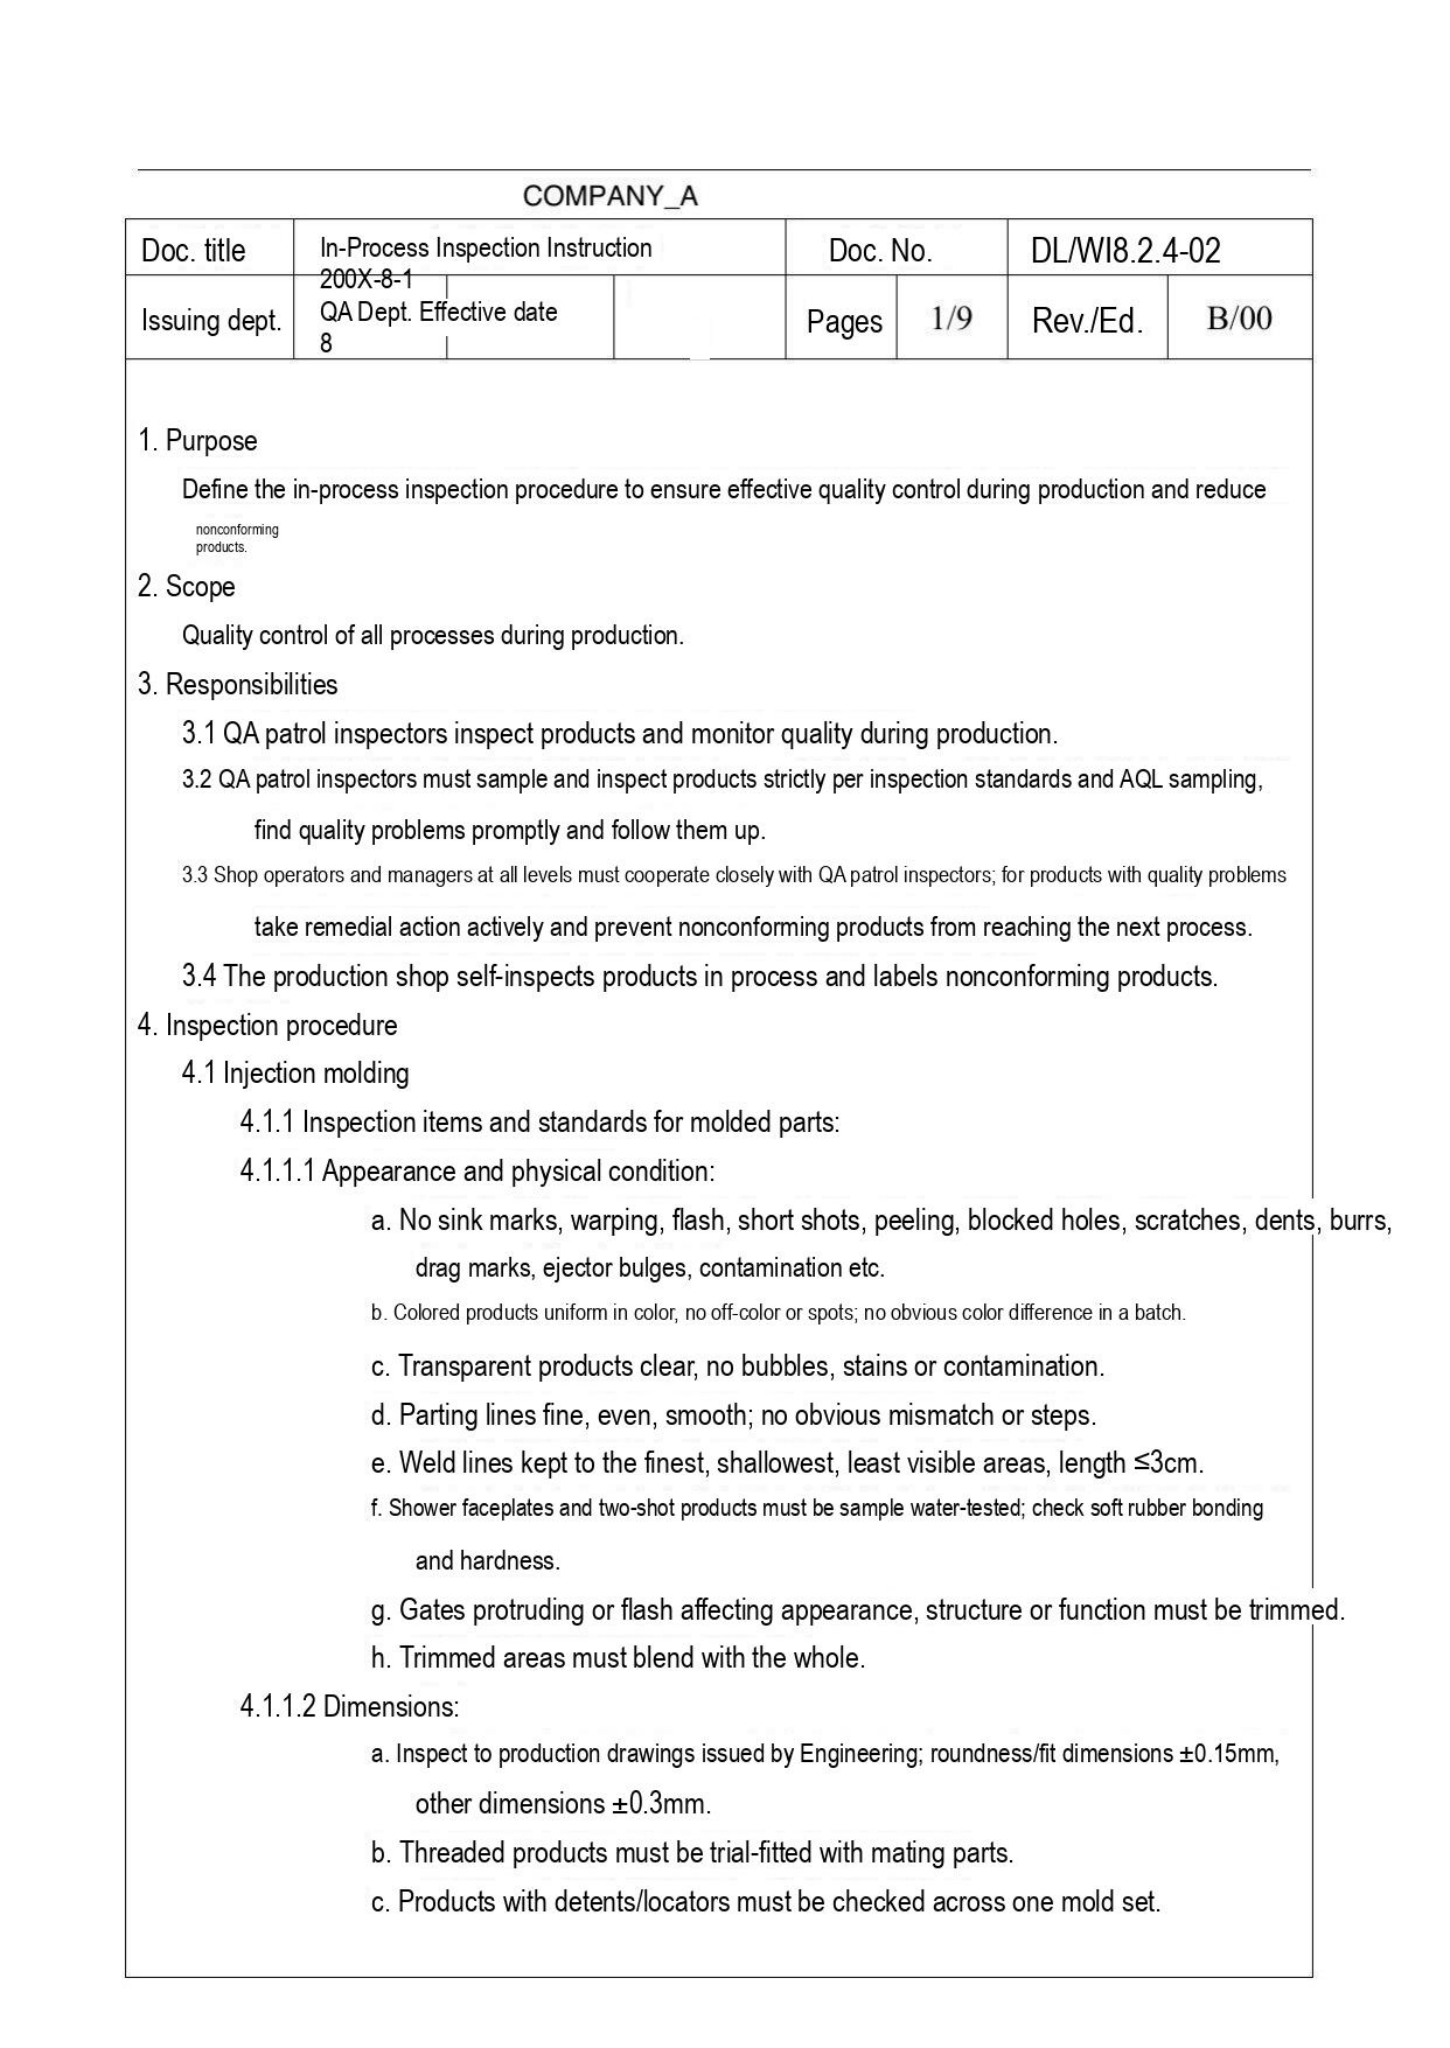COMPANY_A

| Doc. title | In-Process Inspection Instruction | | Doc. No. | DL/WI8.2.4-02 | |
|---|---|---|---|---|---|
| Issuing dept. | 200X-8-1<br>QA Dept. Effective date<br>8 | | Pages 1/9 | Rev./Ed. | B/00 |

1. Purpose

Define the in-process inspection procedure to ensure effective quality control during production and reduce nonconforming products.

2. Scope

Quality control of all processes during production.

3. Responsibilities

3.1 QA patrol inspectors inspect products and monitor quality during production.

3.2 QA patrol inspectors must sample and inspect products strictly per inspection standards and AQL sampling, find quality problems promptly and follow them up.

3.3 Shop operators and managers at all levels must cooperate closely with QA patrol inspectors; for products with quality problems take remedial action actively and prevent nonconforming products from reaching the next process.

3.4 The production shop self-inspects products in process and labels nonconforming products.

4. Inspection procedure

4.1 Injection molding

4.1.1 Inspection items and standards for molded parts:

4.1.1.1 Appearance and physical condition:

a. No sink marks, warping, flash, short shots, peeling, blocked holes, scratches, dents, burrs, drag marks, ejector bulges, contamination etc.

b. Colored products uniform in color, no off-color or spots; no obvious color difference in a batch.

c. Transparent products clear, no bubbles, stains or contamination.

d. Parting lines fine, even, smooth; no obvious mismatch or steps.

e. Weld lines kept to the finest, shallowest, least visible areas, length ≤3cm.

f. Shower faceplates and two-shot products must be sample water-tested; check soft rubber bonding and hardness.

g. Gates protruding or flash affecting appearance, structure or function must be trimmed.

h. Trimmed areas must blend with the whole.

4.1.1.2 Dimensions:

a. Inspect to production drawings issued by Engineering; roundness/fit dimensions ±0.15mm, other dimensions ±0.3mm.

b. Threaded products must be trial-fitted with mating parts.

c. Products with detents/locators must be checked across one mold set.
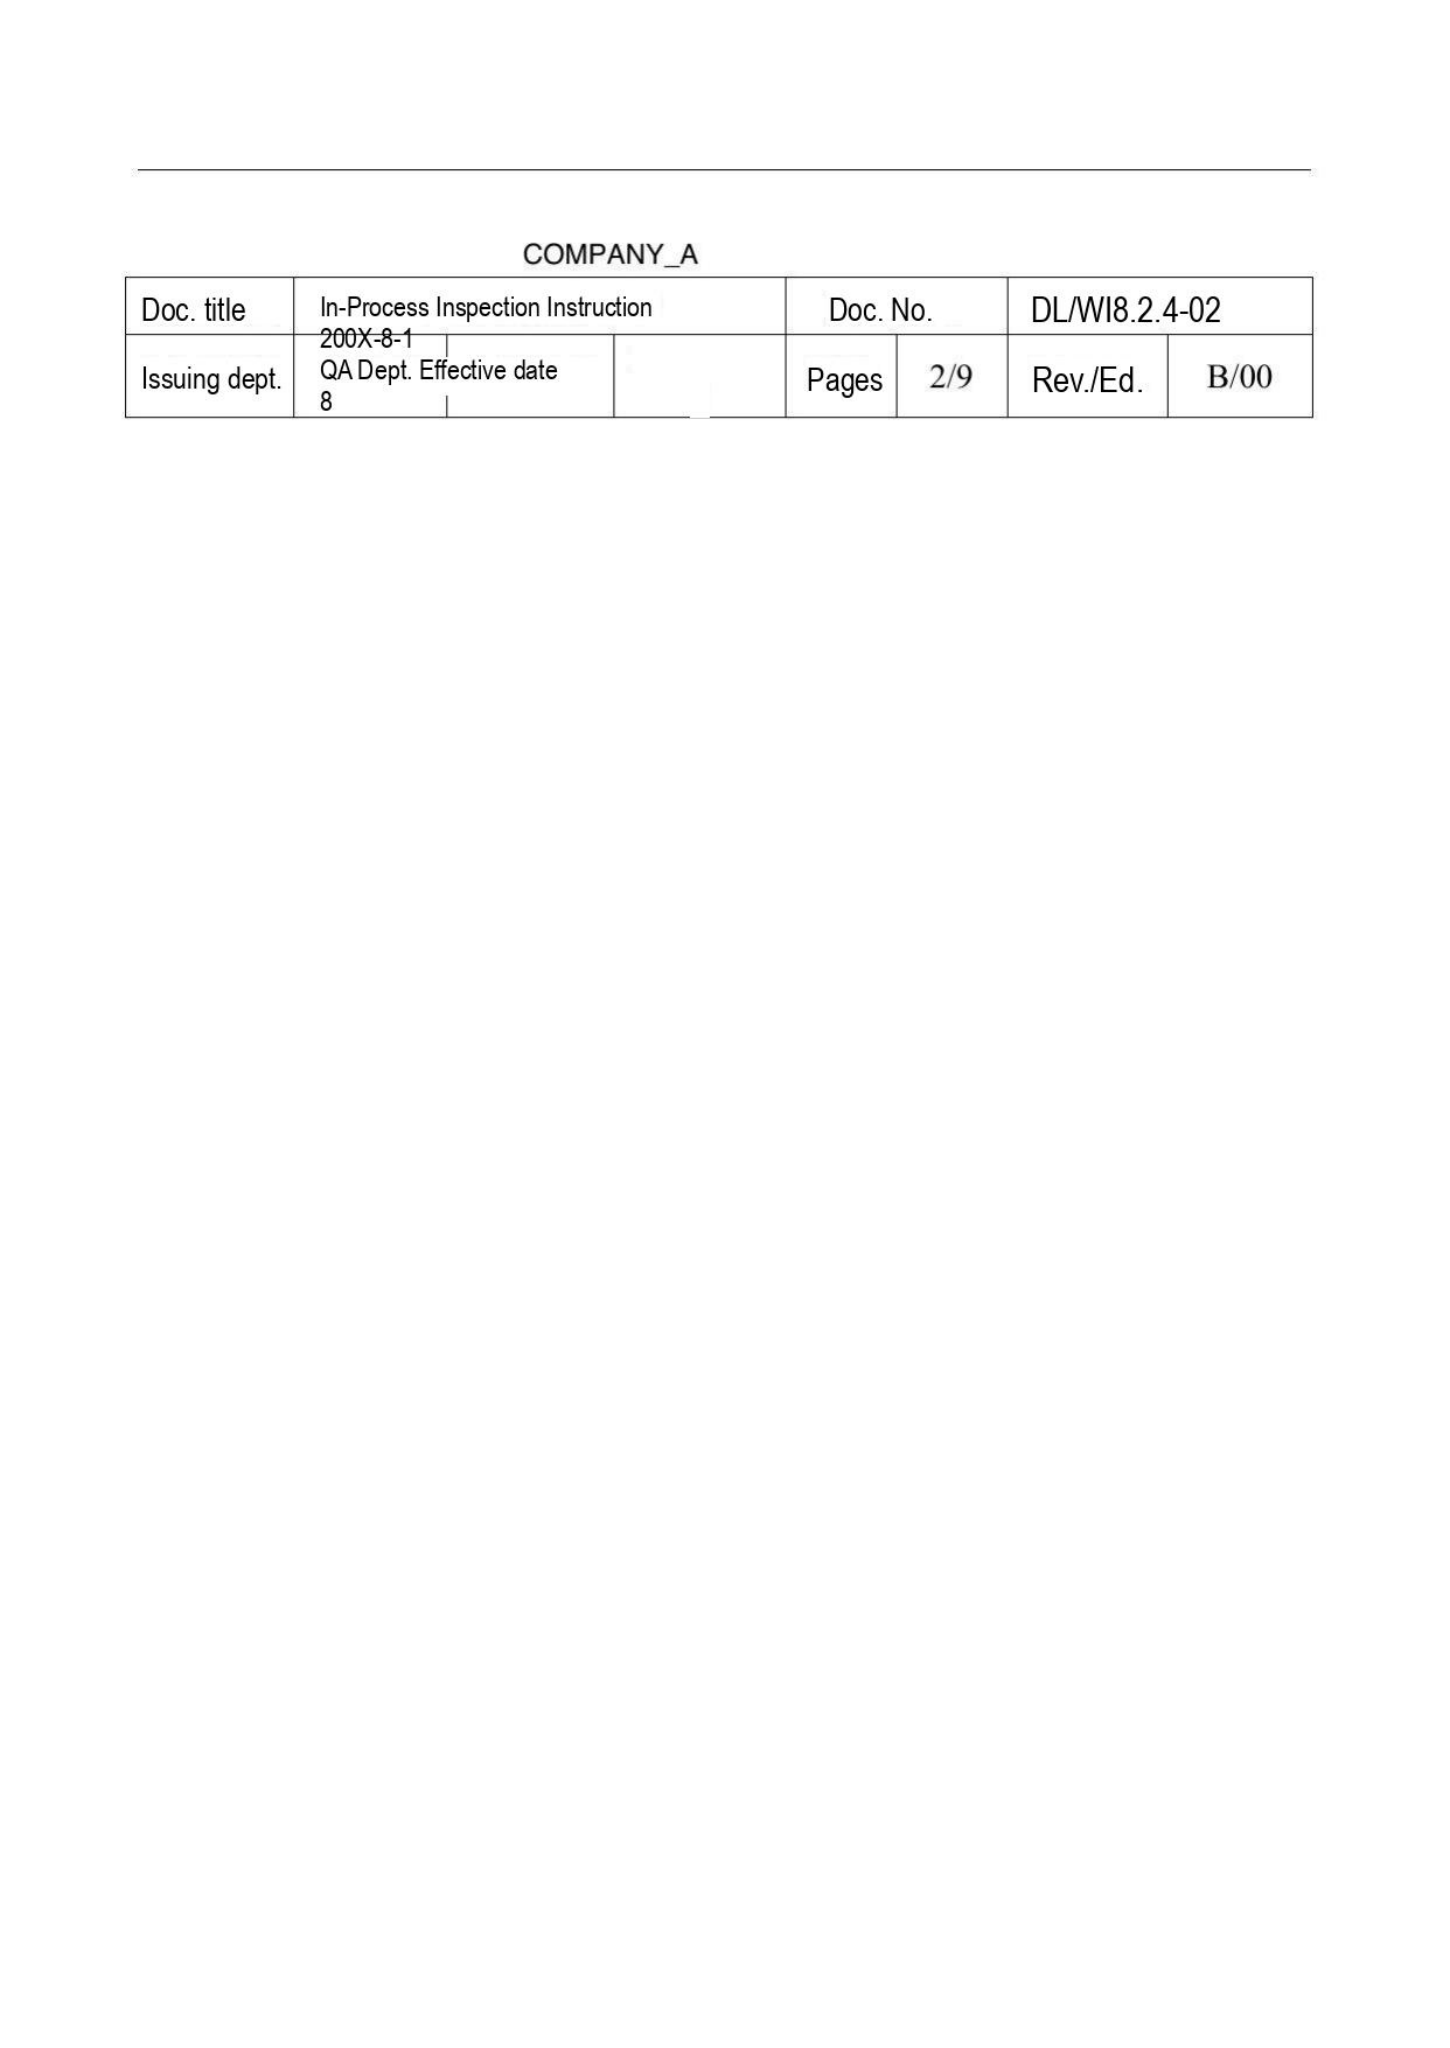COMPANY_A

| Doc. title | In-Process Inspection Instruction | | Doc. No. | DL/WI8.2.4-02 | |
|---|---|---|---|---|---|
| Issuing dept. | 200X-8-1<br>QA Dept. Effective date<br>8 | | Pages | 2/9 | Rev./Ed. | B/00 |
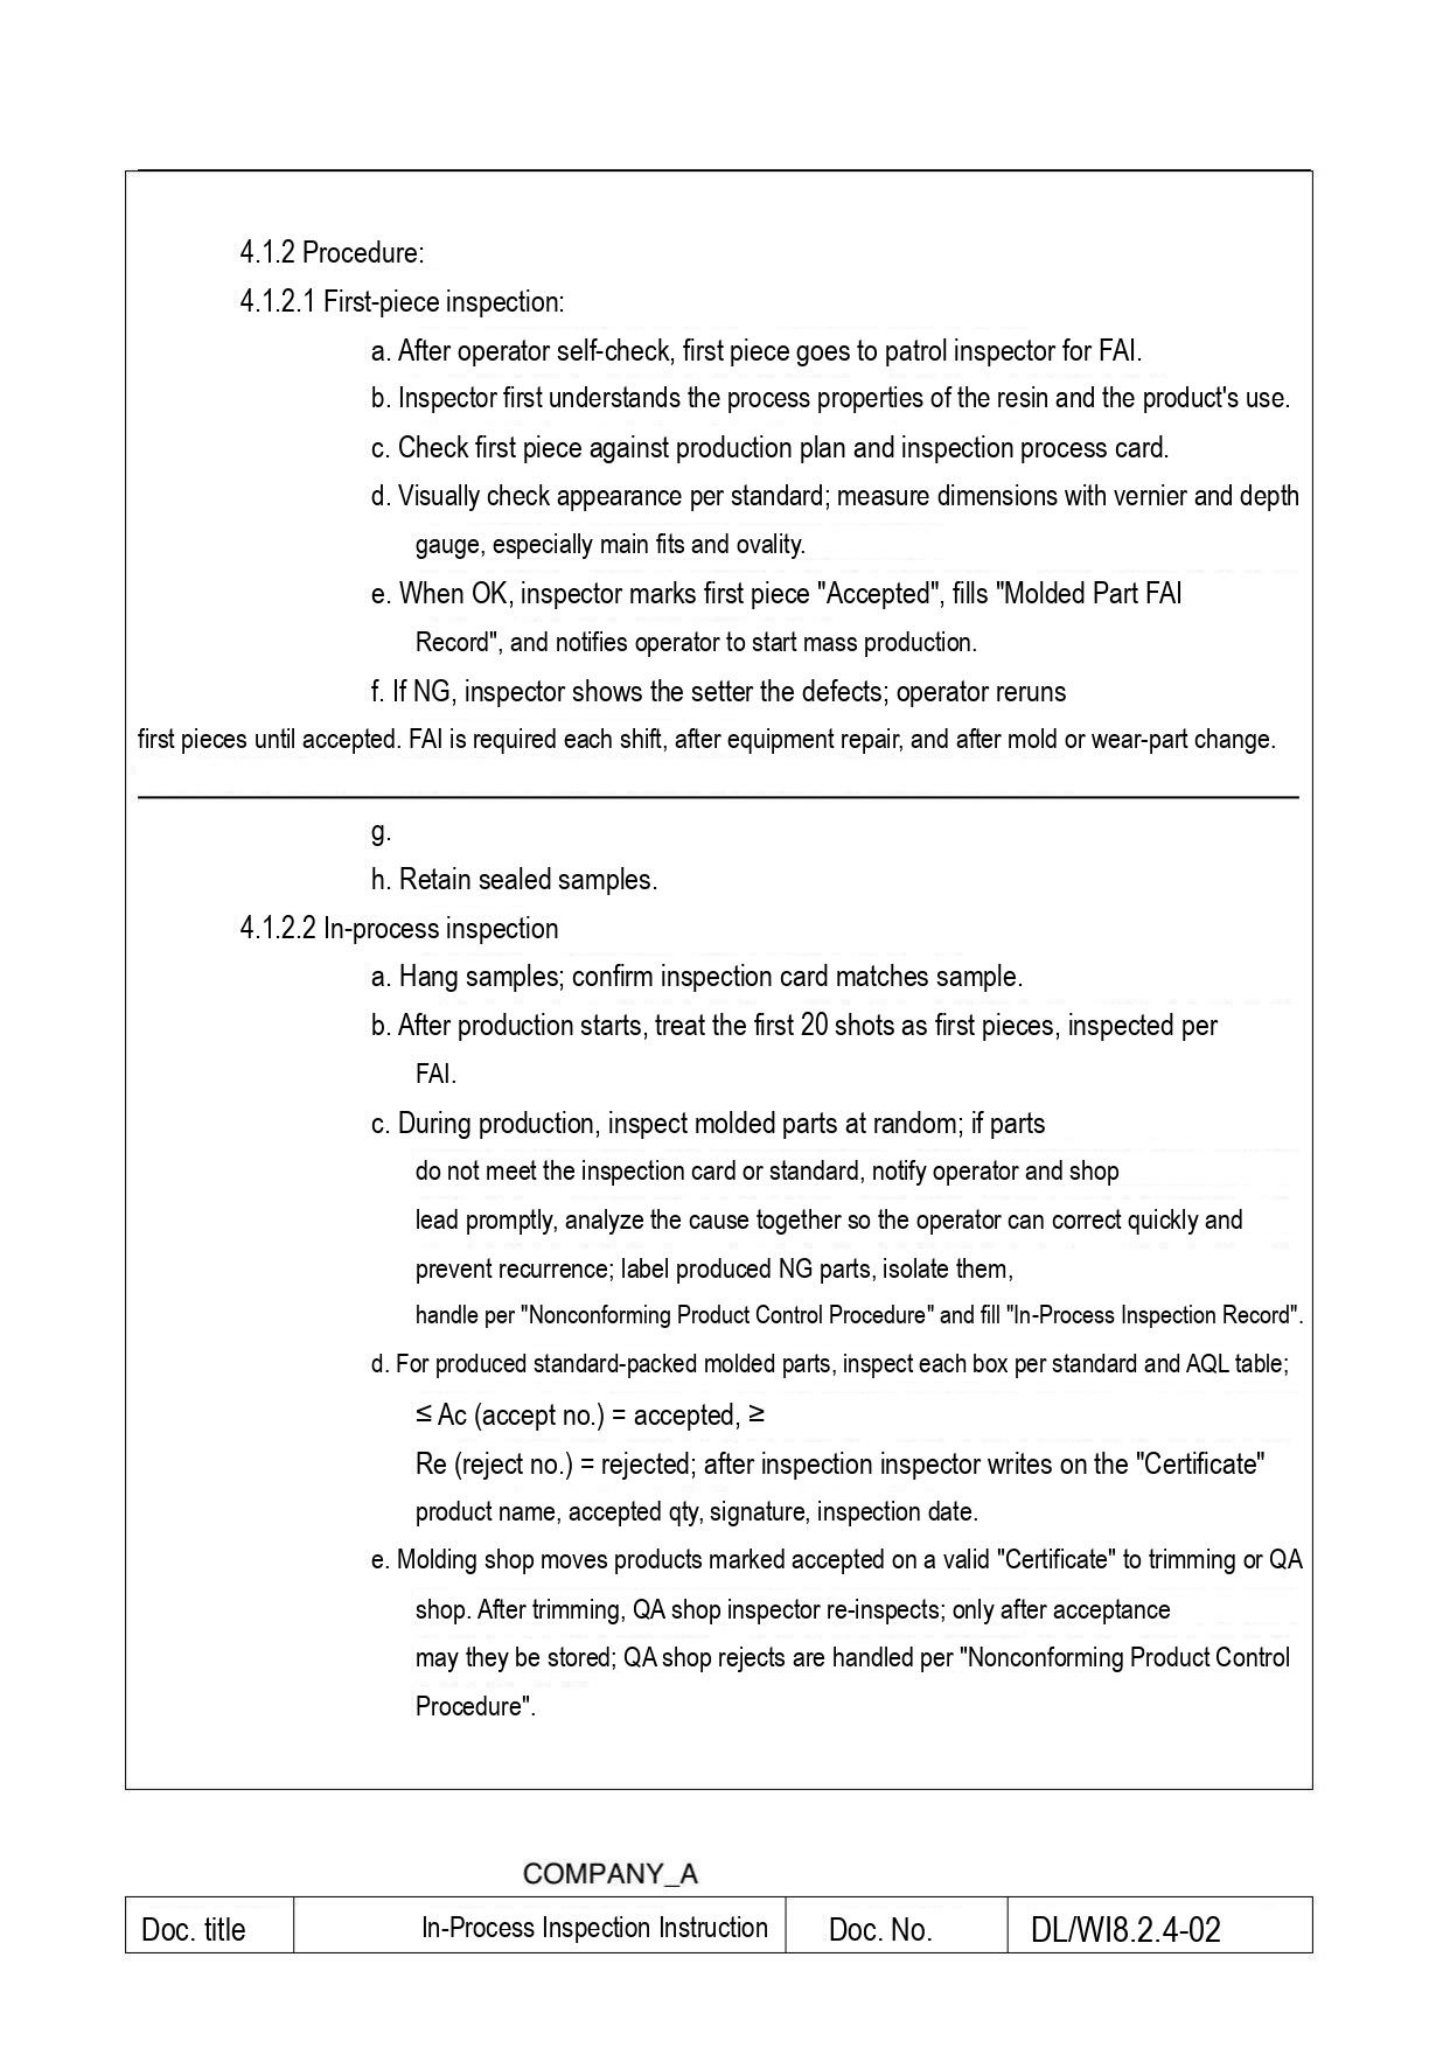4.1.2 Procedure:

4.1.2.1 First-piece inspection:

a. After operator self-check, first piece goes to patrol inspector for FAI.

b. Inspector first understands the process properties of the resin and the product's use.

c. Check first piece against production plan and inspection process card.

d. Visually check appearance per standard; measure dimensions with vernier and depth gauge, especially main fits and ovality.

e. When OK, inspector marks first piece "Accepted", fills "Molded Part FAI Record", and notifies operator to start mass production.

f. If NG, inspector shows the setter the defects; operator reruns first pieces until accepted. FAI is required each shift, after equipment repair, and after mold or wear-part change.

g.

h. Retain sealed samples.

4.1.2.2 In-process inspection

a. Hang samples; confirm inspection card matches sample.

b. After production starts, treat the first 20 shots as first pieces, inspected per FAI.

c. During production, inspect molded parts at random; if parts do not meet the inspection card or standard, notify operator and shop lead promptly, analyze the cause together so the operator can correct quickly and prevent recurrence; label produced NG parts, isolate them, handle per "Nonconforming Product Control Procedure" and fill "In-Process Inspection Record".

d. For produced standard-packed molded parts, inspect each box per standard and AQL table; ≤ Ac (accept no.) = accepted, ≥ Re (reject no.) = rejected; after inspection inspector writes on the "Certificate" product name, accepted qty, signature, inspection date.

e. Molding shop moves products marked accepted on a valid "Certificate" to trimming or QA shop. After trimming, QA shop inspector re-inspects; only after acceptance may they be stored; QA shop rejects are handled per "Nonconforming Product Control Procedure".

COMPANY_A

| Doc. title | In-Process Inspection Instruction | Doc. No. | DL/WI8.2.4-02 |
|---|---|---|---|
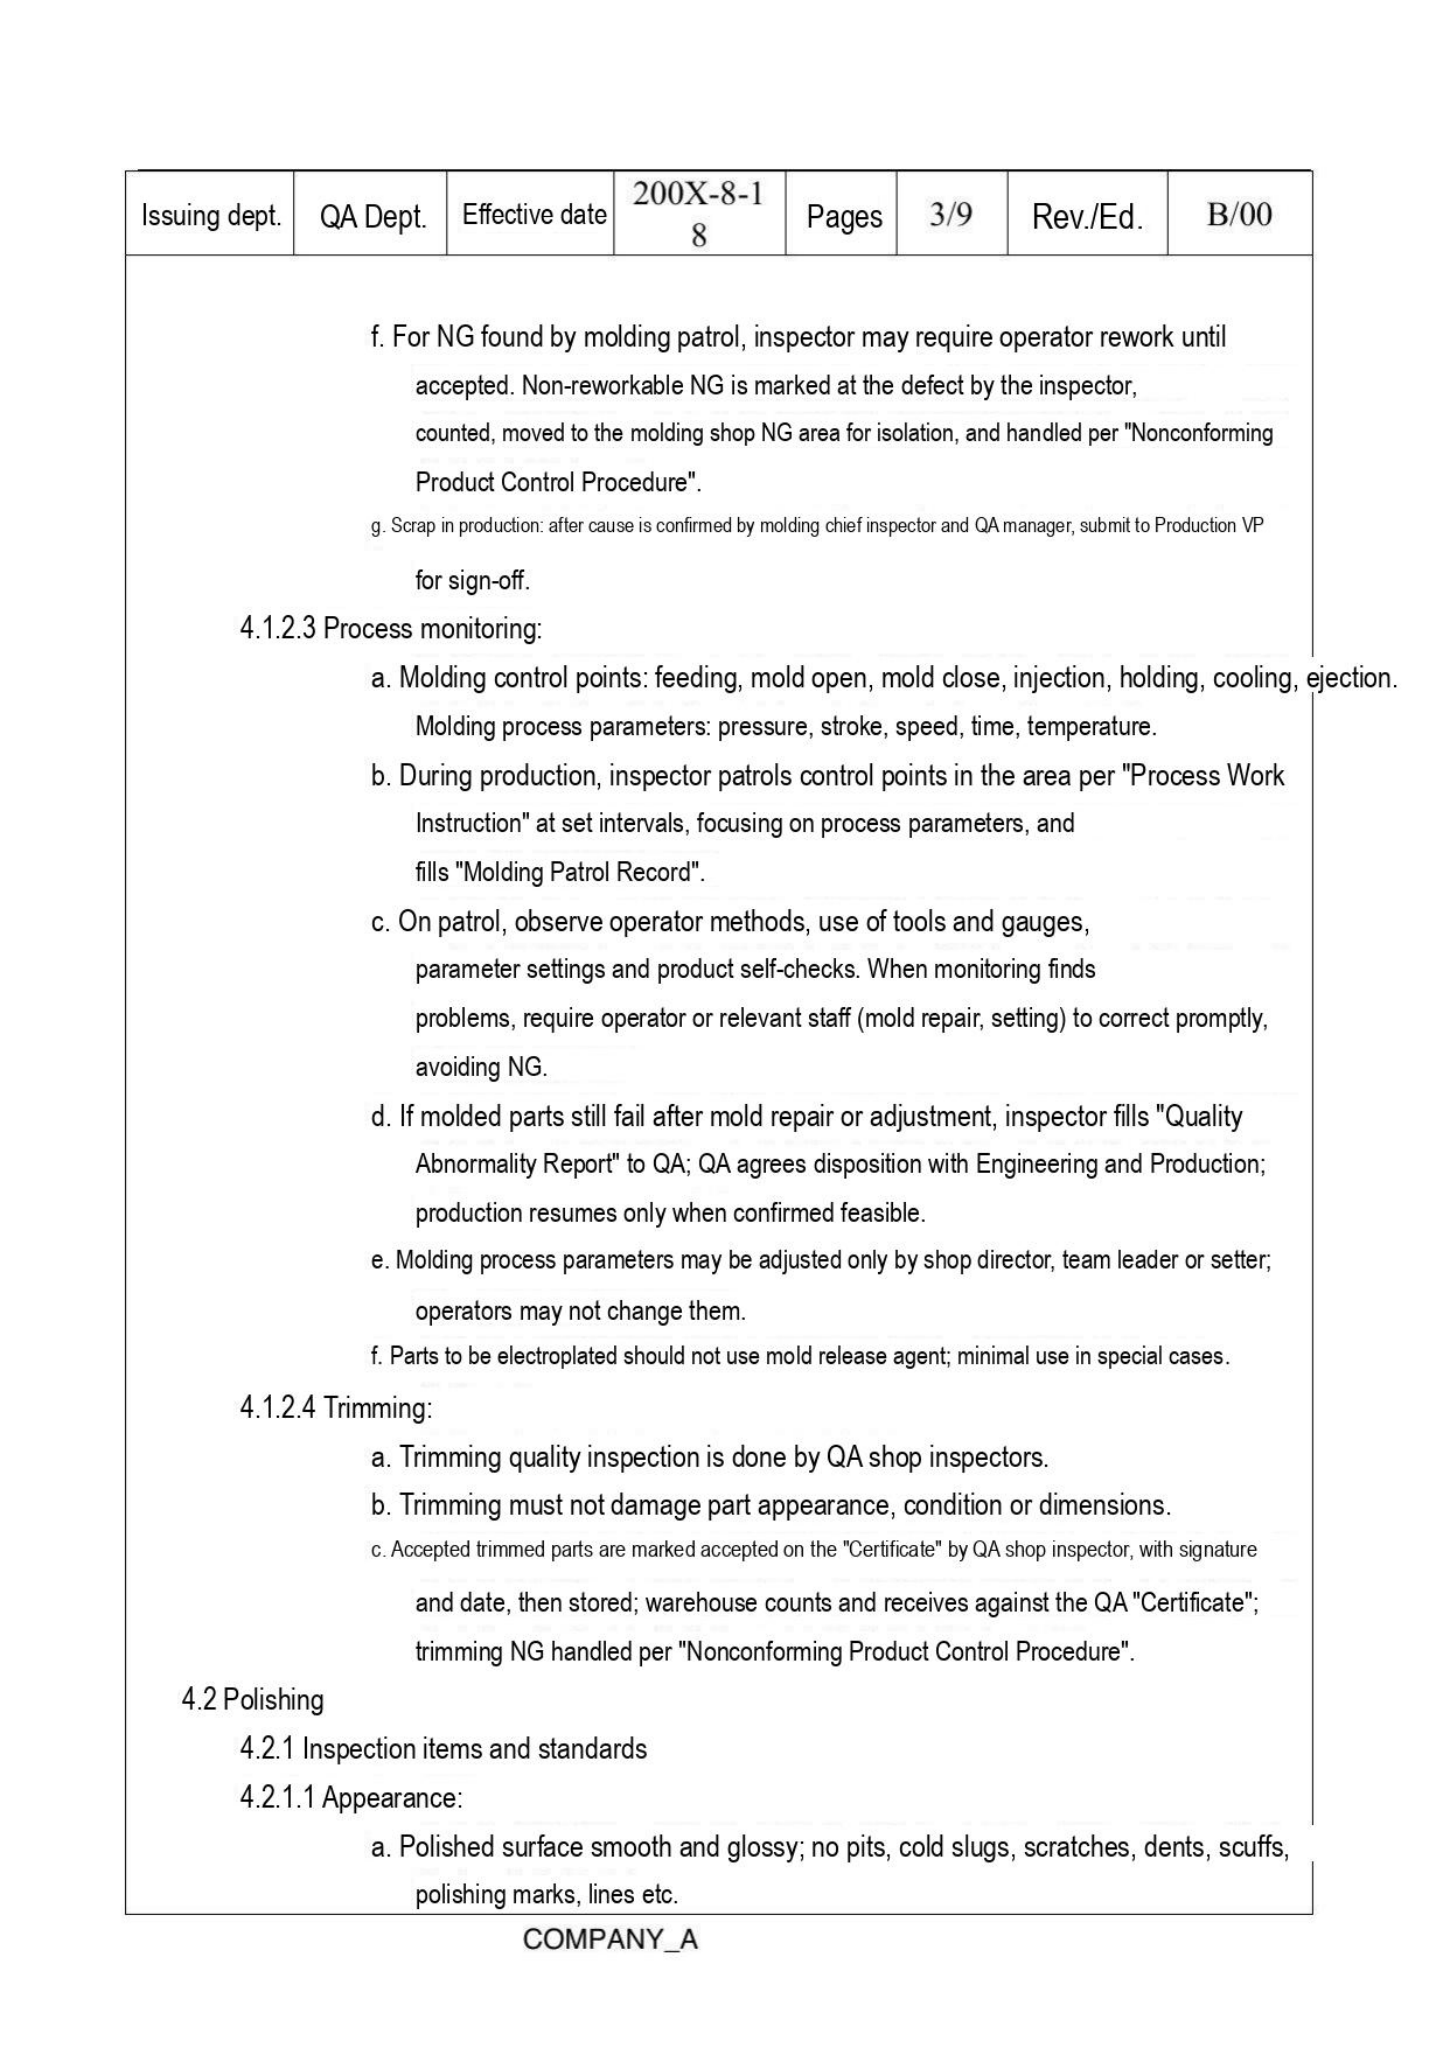| Issuing dept. | QA Dept. | Effective date | 200X-8-18 | Pages | 3/9 | Rev./Ed. | B/00 |
|---|---|---|---|---|---|---|---|

f. For NG found by molding patrol, inspector may require operator rework until accepted. Non-reworkable NG is marked at the defect by the inspector, counted, moved to the molding shop NG area for isolation, and handled per "Nonconforming Product Control Procedure".

g. Scrap in production: after cause is confirmed by molding chief inspector and QA manager, submit to Production VP for sign-off.

4.1.2.3 Process monitoring:

a. Molding control points: feeding, mold open, mold close, injection, holding, cooling, ejection. Molding process parameters: pressure, stroke, speed, time, temperature.

b. During production, inspector patrols control points in the area per "Process Work Instruction" at set intervals, focusing on process parameters, and fills "Molding Patrol Record".

c. On patrol, observe operator methods, use of tools and gauges, parameter settings and product self-checks. When monitoring finds problems, require operator or relevant staff (mold repair, setting) to correct promptly, avoiding NG.

d. If molded parts still fail after mold repair or adjustment, inspector fills "Quality Abnormality Report" to QA; QA agrees disposition with Engineering and Production; production resumes only when confirmed feasible.

e. Molding process parameters may be adjusted only by shop director, team leader or setter; operators may not change them.

f. Parts to be electroplated should not use mold release agent; minimal use in special cases.

4.1.2.4 Trimming:

a. Trimming quality inspection is done by QA shop inspectors.

b. Trimming must not damage part appearance, condition or dimensions.

c. Accepted trimmed parts are marked accepted on the "Certificate" by QA shop inspector, with signature and date, then stored; warehouse counts and receives against the QA "Certificate"; trimming NG handled per "Nonconforming Product Control Procedure".

4.2 Polishing

4.2.1 Inspection items and standards

4.2.1.1 Appearance:

a. Polished surface smooth and glossy; no pits, cold slugs, scratches, dents, scuffs, polishing marks, lines etc.

COMPANY_A
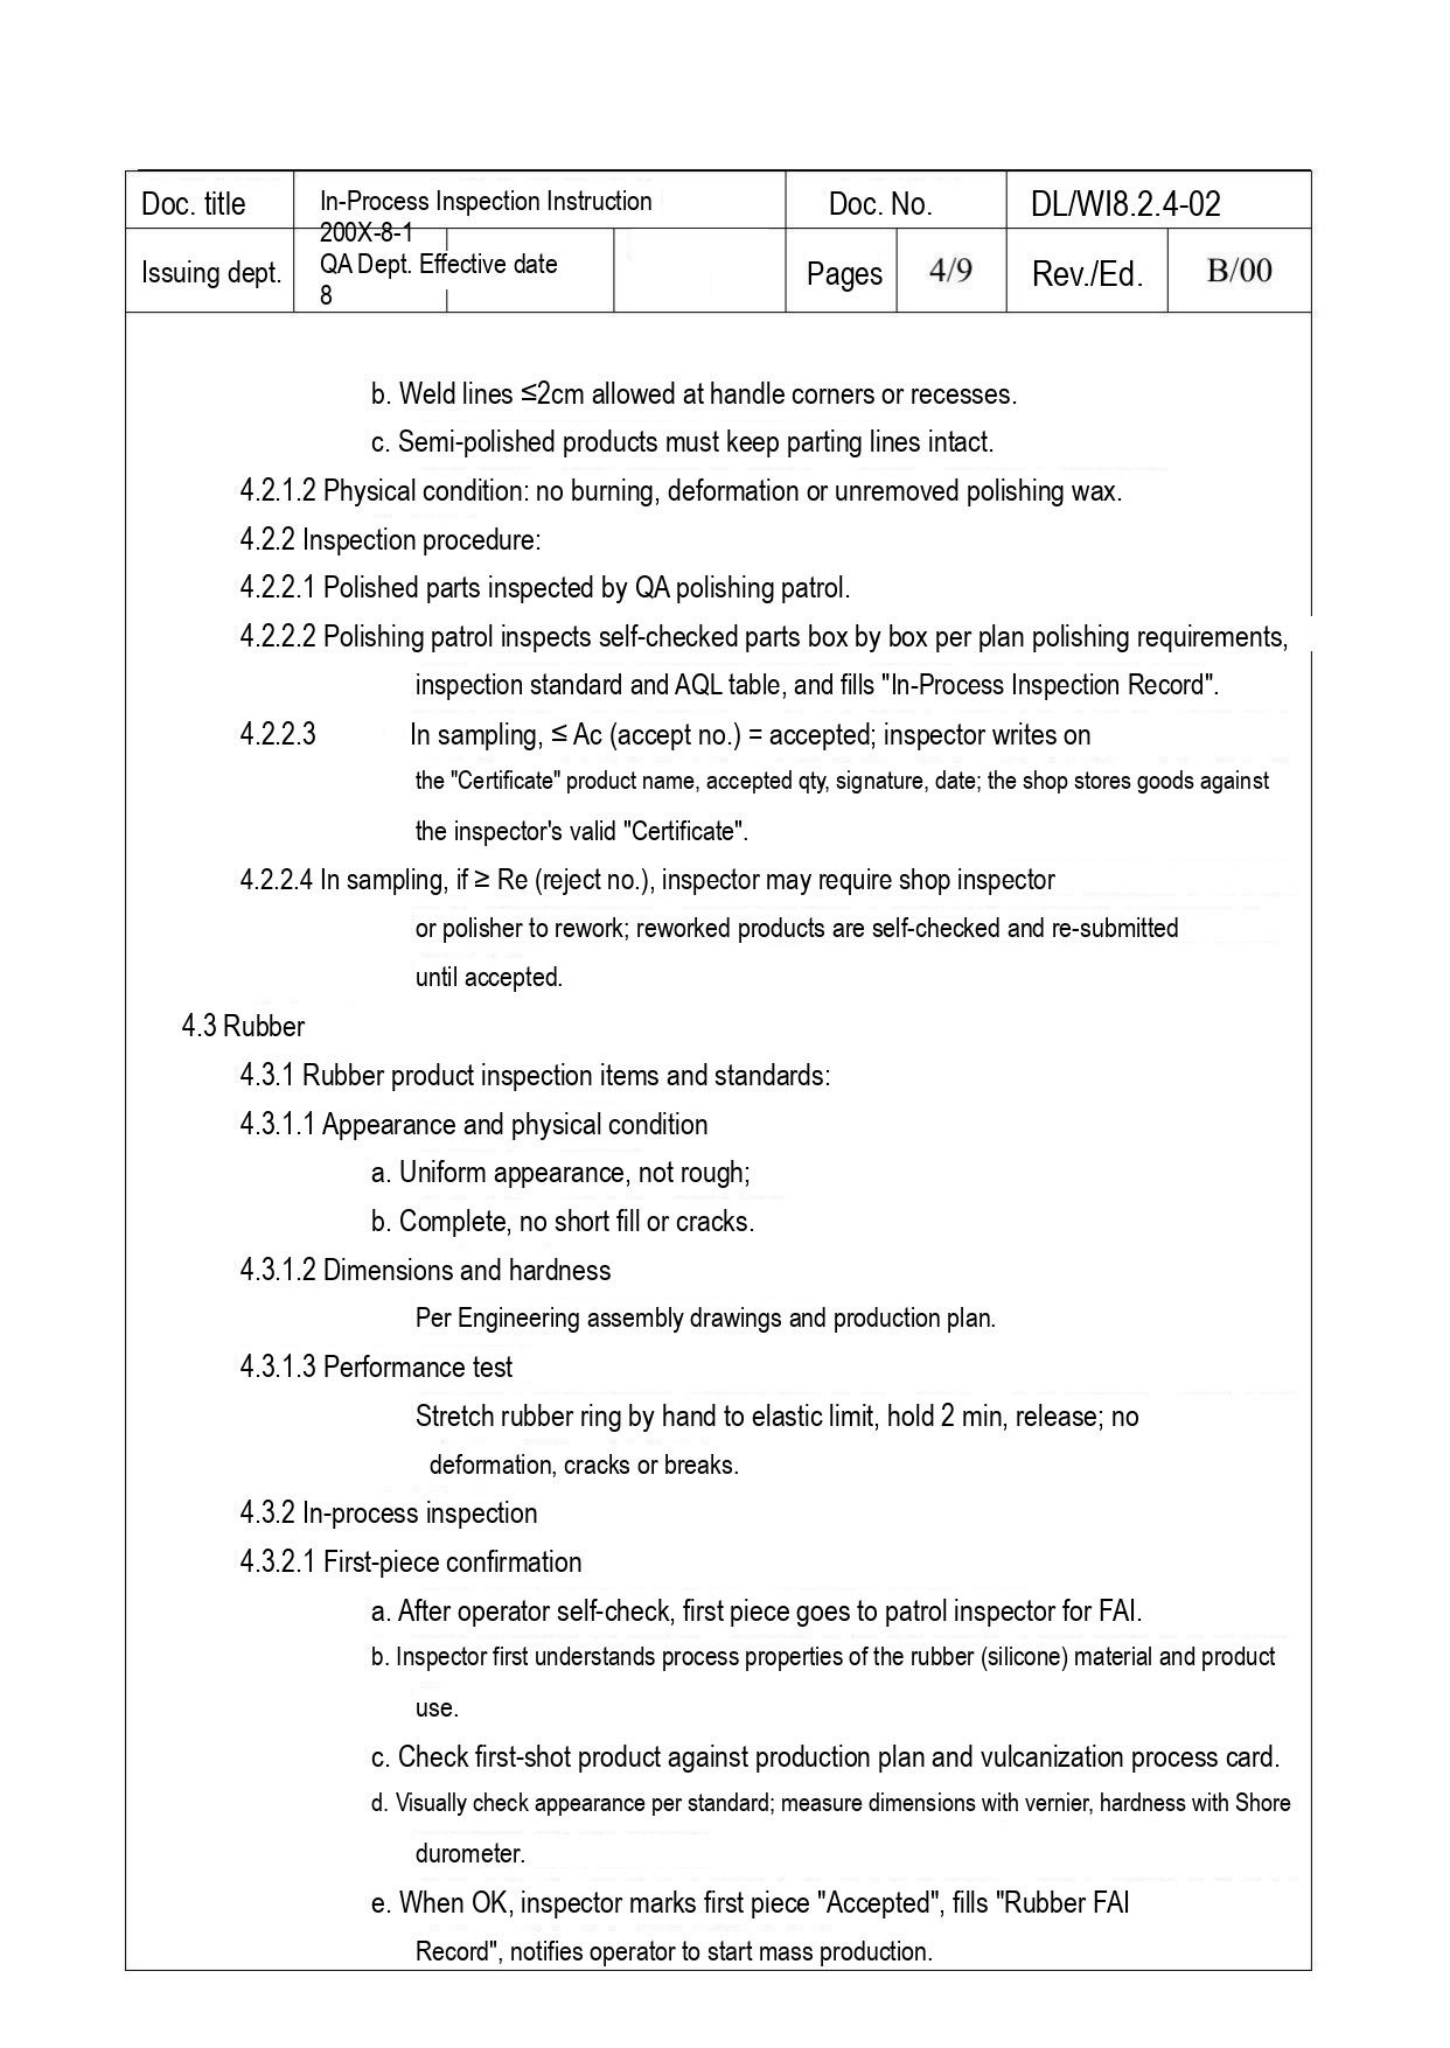| Doc. title | In-Process Inspection Instruction | Doc. No. | DL/WI8.2.4-02 |
|---|---|---|---|
| Issuing dept. | 200X-8-1 QA Dept. Effective date 8 | Pages 4/9 | Rev./Ed. B/00 |

b. Weld lines ≤2cm allowed at handle corners or recesses.

c. Semi-polished products must keep parting lines intact.

4.2.1.2 Physical condition: no burning, deformation or unremoved polishing wax.

4.2.2 Inspection procedure:

4.2.2.1 Polished parts inspected by QA polishing patrol.

4.2.2.2 Polishing patrol inspects self-checked parts box by box per plan polishing requirements, inspection standard and AQL table, and fills "In-Process Inspection Record".

4.2.2.3 In sampling, ≤ Ac (accept no.) = accepted; inspector writes on the "Certificate" product name, accepted qty, signature, date; the shop stores goods against the inspector's valid "Certificate".

4.2.2.4 In sampling, if ≥ Re (reject no.), inspector may require shop inspector or polisher to rework; reworked products are self-checked and re-submitted until accepted.

4.3 Rubber

4.3.1 Rubber product inspection items and standards:

4.3.1.1 Appearance and physical condition

a. Uniform appearance, not rough;

b. Complete, no short fill or cracks.

4.3.1.2 Dimensions and hardness

Per Engineering assembly drawings and production plan.

4.3.1.3 Performance test

Stretch rubber ring by hand to elastic limit, hold 2 min, release; no deformation, cracks or breaks.

4.3.2 In-process inspection

4.3.2.1 First-piece confirmation

a. After operator self-check, first piece goes to patrol inspector for FAI.

b. Inspector first understands process properties of the rubber (silicone) material and product use.

c. Check first-shot product against production plan and vulcanization process card.

d. Visually check appearance per standard; measure dimensions with vernier, hardness with Shore durometer.

e. When OK, inspector marks first piece "Accepted", fills "Rubber FAI Record", notifies operator to start mass production.
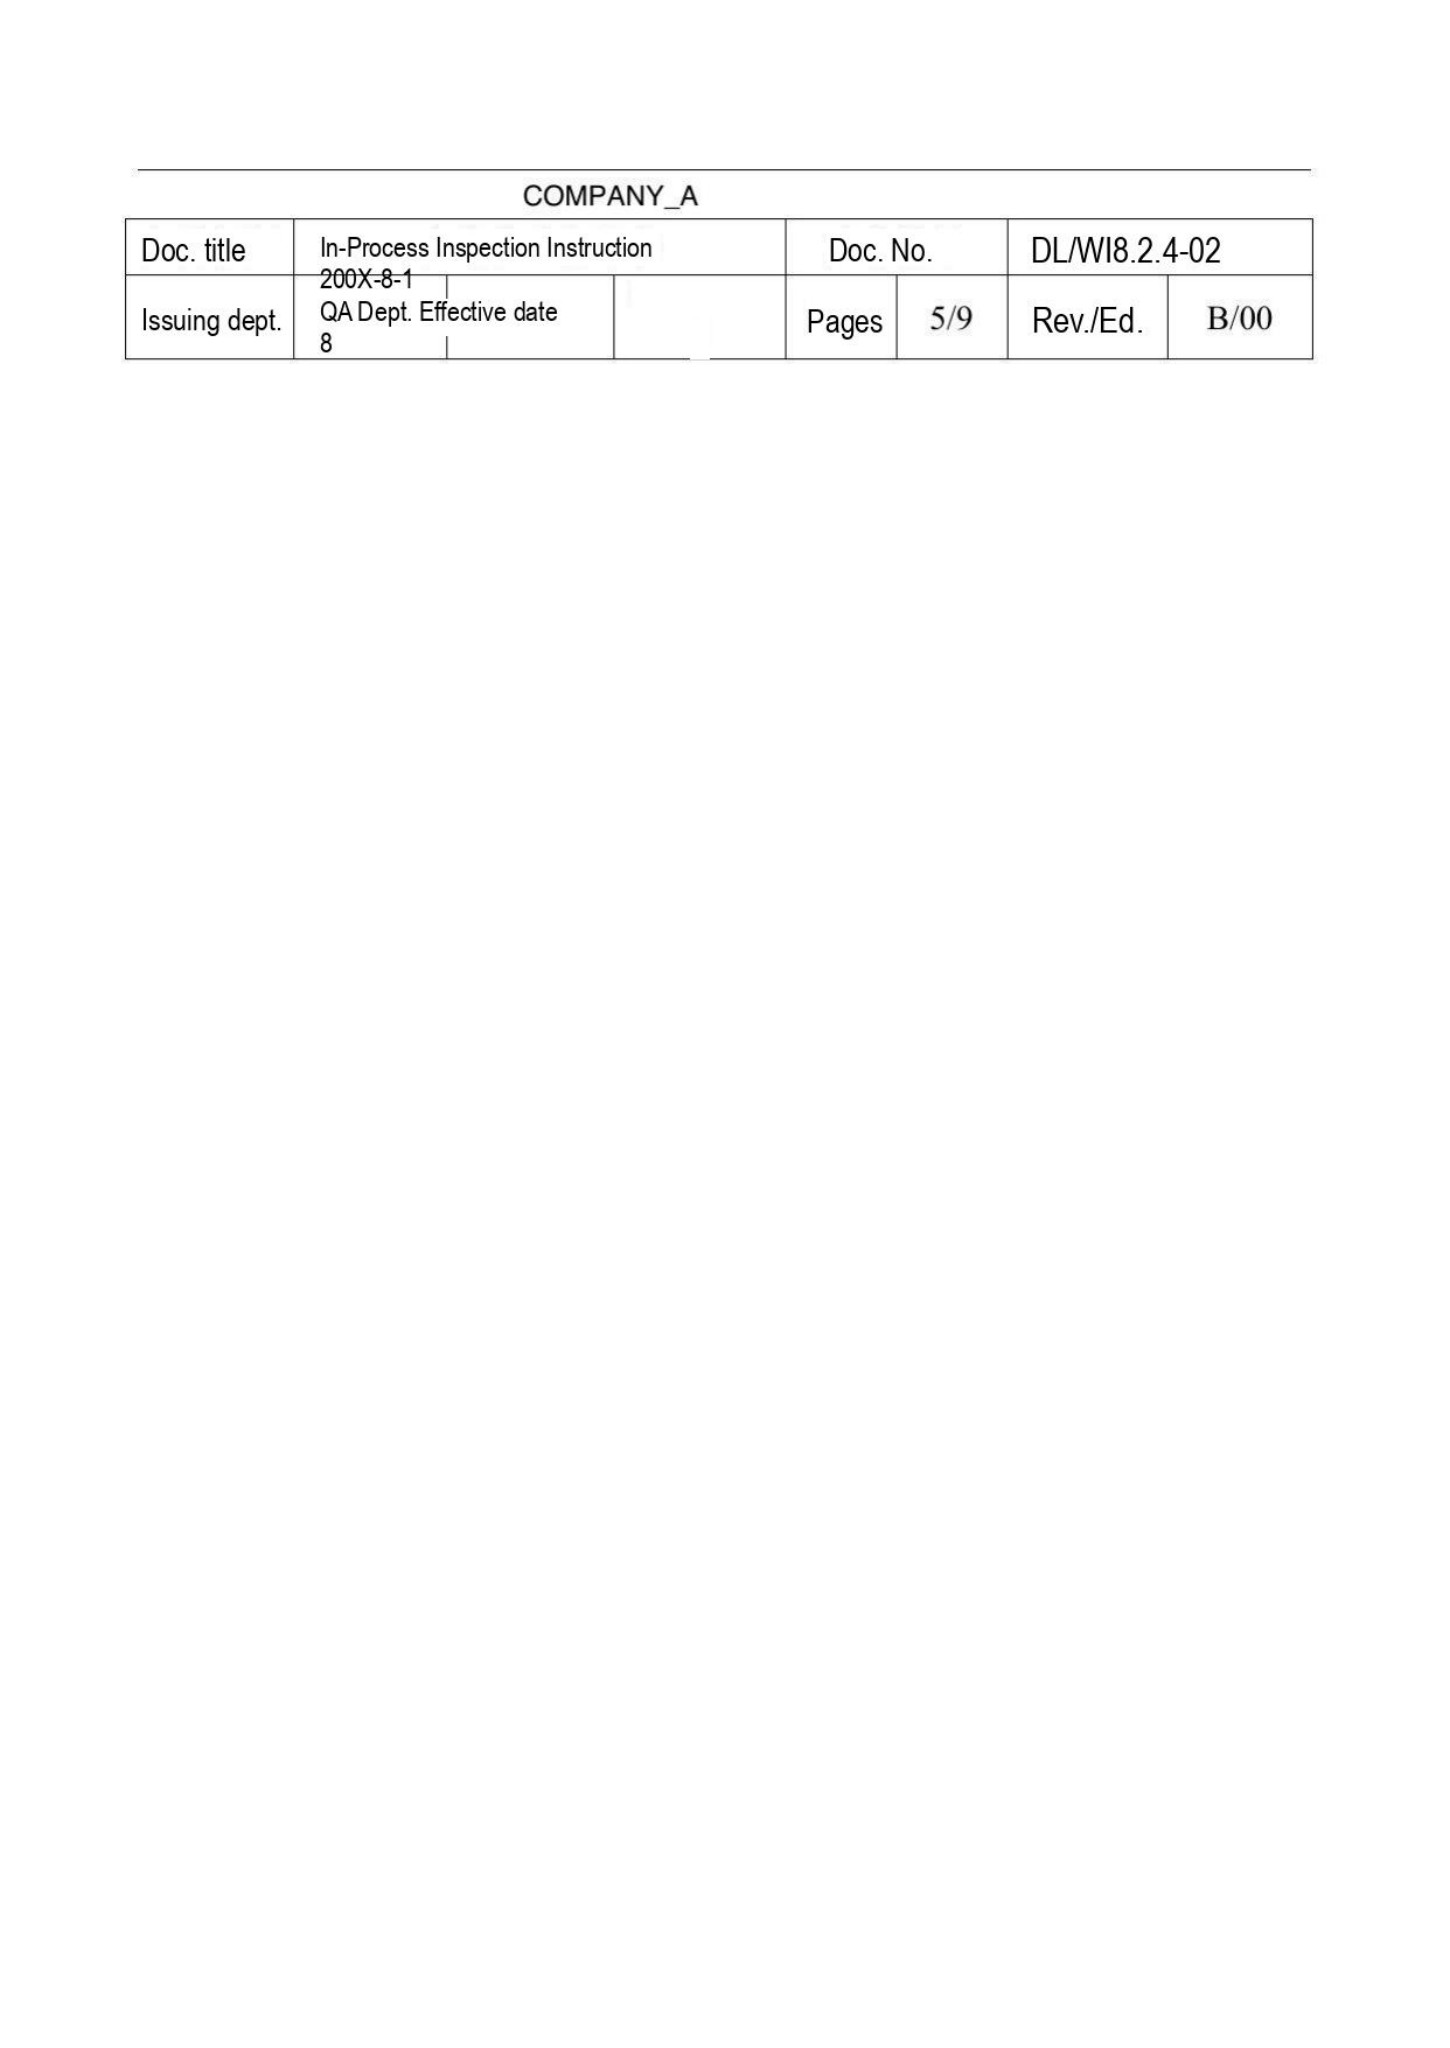COMPANY_A

| Doc. title | In-Process Inspection Instruction | | Doc. No. | DL/WI8.2.4-02 | |
|---|---|---|---|---|---|
| Issuing dept. | 200X-8-1 QA Dept. Effective date 8 | Pages | 5/9 | Rev./Ed. | B/00 |
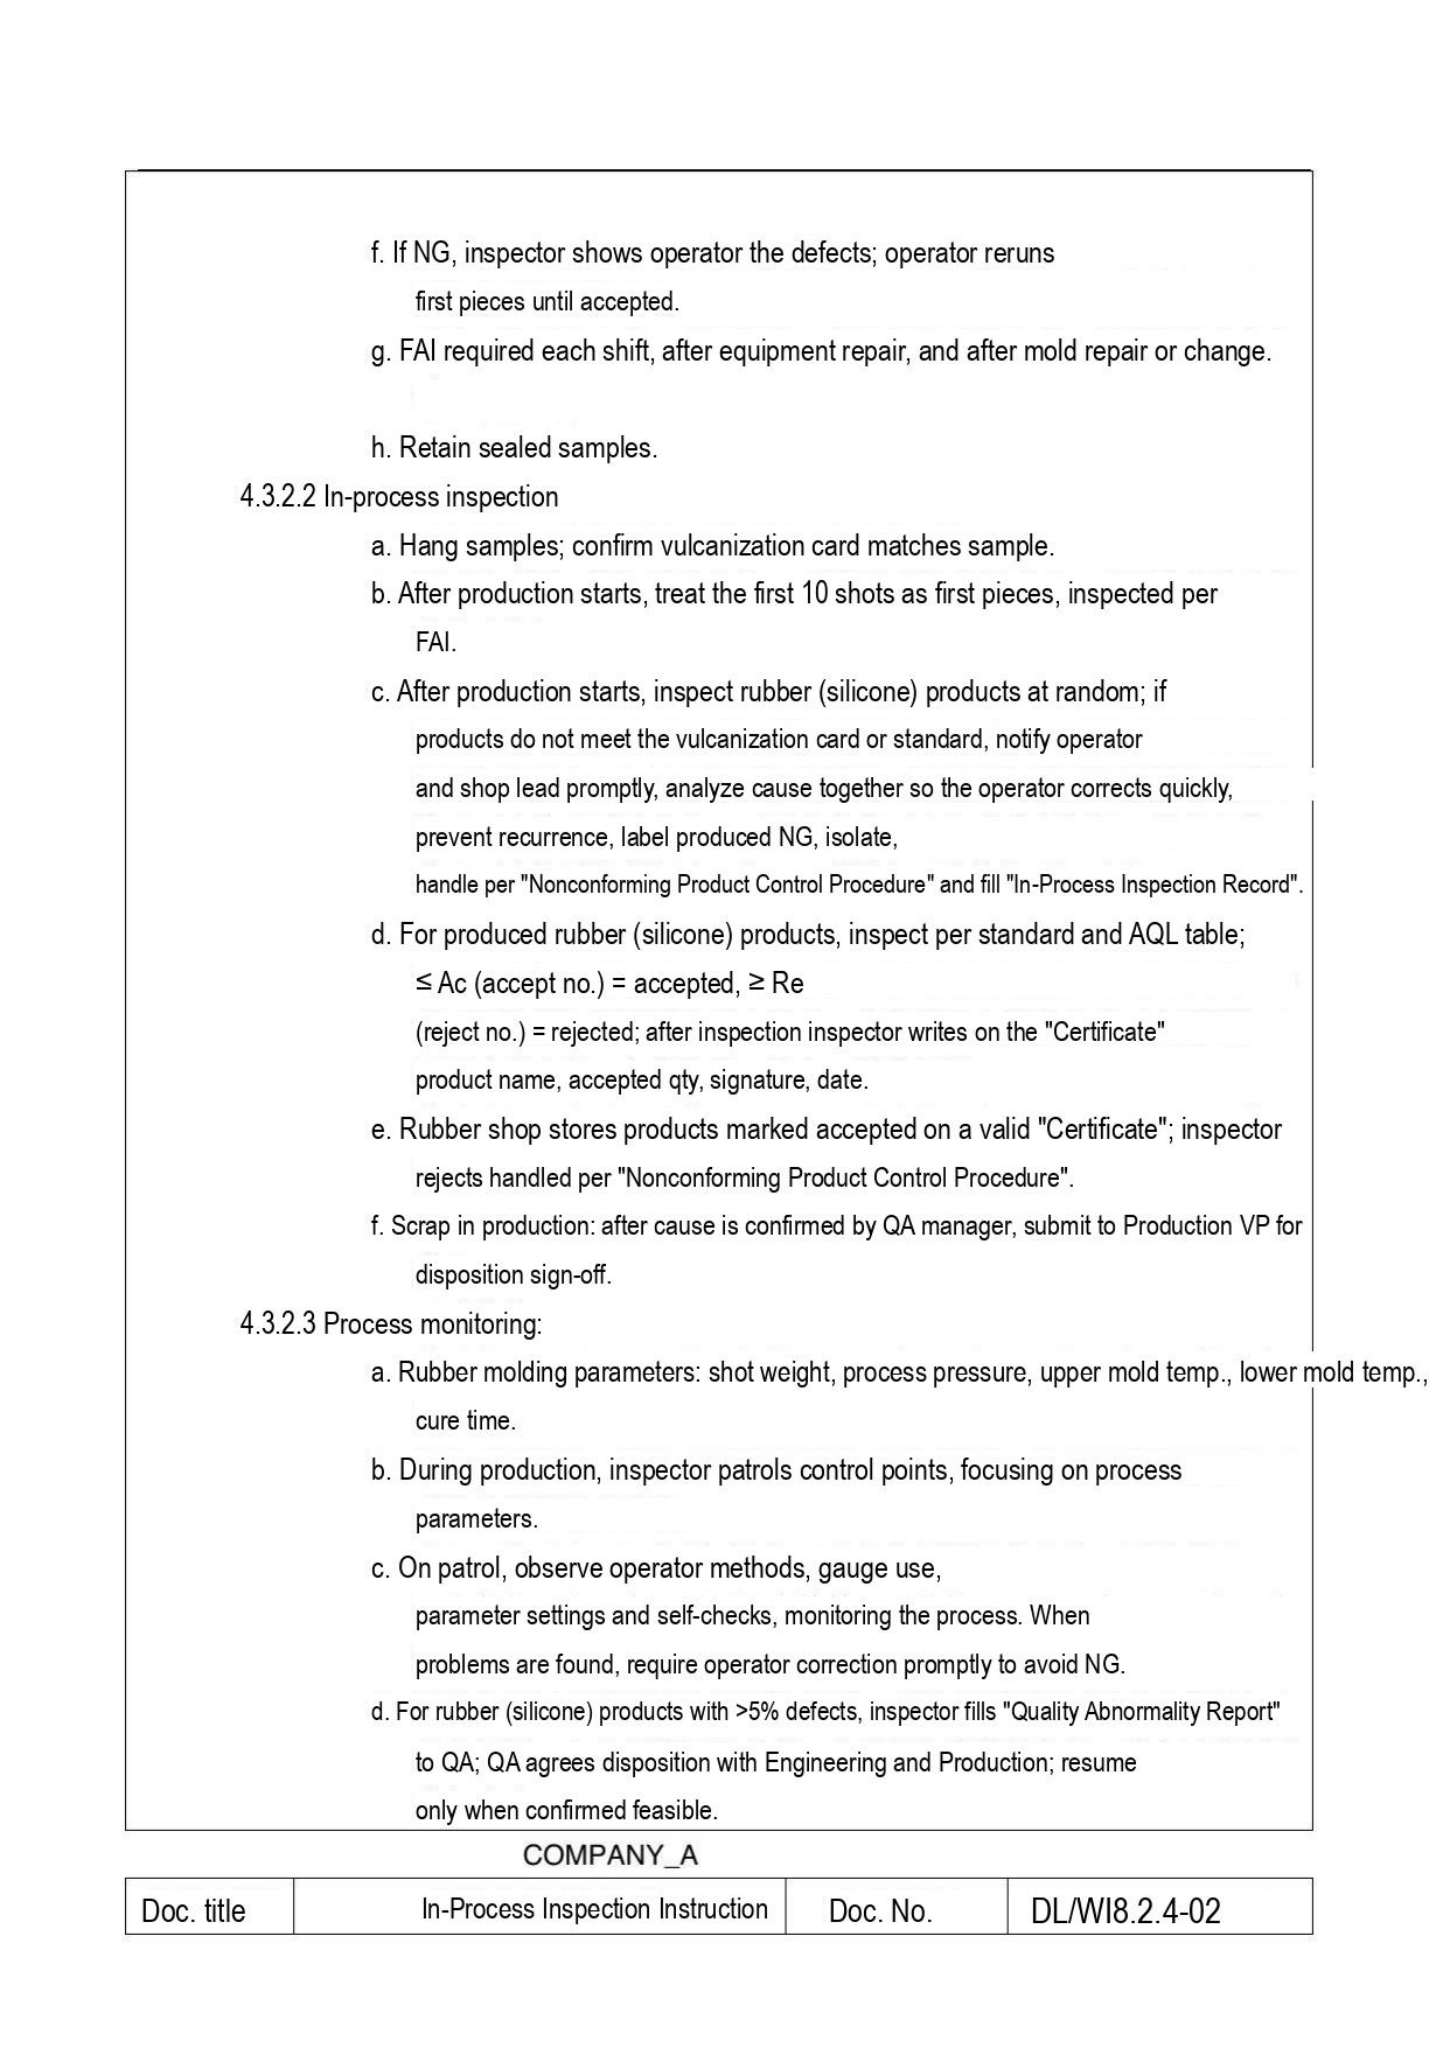f. If NG, inspector shows operator the defects; operator reruns first pieces until accepted.

g. FAI required each shift, after equipment repair, and after mold repair or change.

h. Retain sealed samples.

4.3.2.2 In-process inspection

a. Hang samples; confirm vulcanization card matches sample.

b. After production starts, treat the first 10 shots as first pieces, inspected per FAI.

c. After production starts, inspect rubber (silicone) products at random; if products do not meet the vulcanization card or standard, notify operator and shop lead promptly, analyze cause together so the operator corrects quickly, prevent recurrence, label produced NG, isolate, handle per "Nonconforming Product Control Procedure" and fill "In-Process Inspection Record".

d. For produced rubber (silicone) products, inspect per standard and AQL table; ≤ Ac (accept no.) = accepted, ≥ Re (reject no.) = rejected; after inspection inspector writes on the "Certificate" product name, accepted qty, signature, date.

e. Rubber shop stores products marked accepted on a valid "Certificate"; inspector rejects handled per "Nonconforming Product Control Procedure".

f. Scrap in production: after cause is confirmed by QA manager, submit to Production VP for disposition sign-off.

4.3.2.3 Process monitoring:

a. Rubber molding parameters: shot weight, process pressure, upper mold temp., lower mold temp., cure time.

b. During production, inspector patrols control points, focusing on process parameters.

c. On patrol, observe operator methods, gauge use, parameter settings and self-checks, monitoring the process. When problems are found, require operator correction promptly to avoid NG.

d. For rubber (silicone) products with >5% defects, inspector fills "Quality Abnormality Report" to QA; QA agrees disposition with Engineering and Production; resume only when confirmed feasible.

COMPANY_A

| Doc. title | In-Process Inspection Instruction | Doc. No. | DL/WI8.2.4-02 |
|---|---|---|---|